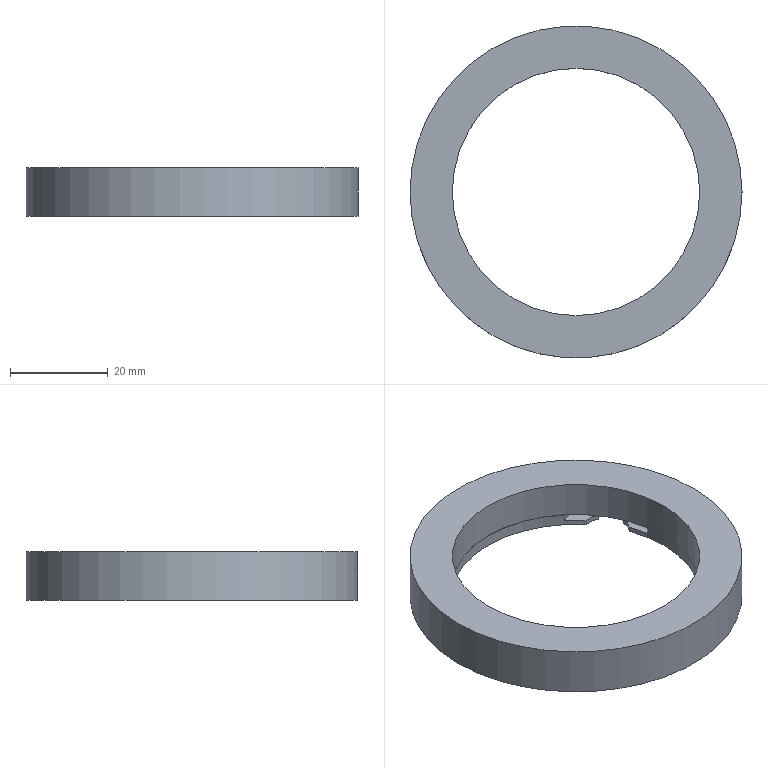Part | STEP file | 1 solid | 31 faces | box 67.8 x 67.8 x 10 mm | volume 15491 mm3 | cylinder 17 | plane 12 | cone 2 | commonest cylinder face diameters 9.7 x4 5.3 x3 17.7 x3 50.7 x3 10 x2 50.5 x1
STEP:
#1=CARTESIAN_POINT('',(-8.838,-23.759,-13.81));
#2=VERTEX_POINT('',#1);
#3=CARTESIAN_POINT('',(-8.838,-23.759,-15.31));
#4=VERTEX_POINT('',#3);
#5=CARTESIAN_POINT('',(-8.838,-23.759,-13.81));
#6=DIRECTION('',(0.,0.,-1.));
#7=VECTOR('',#6,1.);
#8=LINE('',#5,#7);
#9=EDGE_CURVE('',#2,#4,#8,.T.);
#10=ORIENTED_EDGE('',*,*,#9,.F.);
#11=CARTESIAN_POINT('',(8.838,-23.759,-13.81));
#12=VERTEX_POINT('',#11);
#13=CARTESIAN_POINT('',(0.,-23.3,-13.81));
#14=DIRECTION('',(0.,0.,-1.));
#15=DIRECTION('',(0.9987,-0.05191,0.));
#16=AXIS2_PLACEMENT_3D('',#13,#14,#15);
#17=CIRCLE('',#16,8.85);
#18=EDGE_CURVE('',#12,#2,#17,.T.);
#19=ORIENTED_EDGE('',*,*,#18,.F.);
#20=CARTESIAN_POINT('',(8.838,-23.759,-15.31));
#21=VERTEX_POINT('',#20);
#22=CARTESIAN_POINT('',(8.838,-23.759,-15.31));
#23=DIRECTION('',(0.,0.,1.));
#24=VECTOR('',#23,1.);
#25=LINE('',#22,#24);
#26=EDGE_CURVE('',#21,#12,#25,.T.);
#27=ORIENTED_EDGE('',*,*,#26,.F.);
#28=CARTESIAN_POINT('',(0.,-23.3,-15.31));
#29=DIRECTION('',(0.,0.,1.));
#30=DIRECTION('',(-0.9987,-0.05191,0.));
#31=AXIS2_PLACEMENT_3D('',#28,#29,#30);
#32=CIRCLE('',#31,8.85);
#33=EDGE_CURVE('',#4,#21,#32,.T.);
#34=ORIENTED_EDGE('',*,*,#33,.F.);
#35=EDGE_LOOP('',(#10,#19,#27,#34));
#36=FACE_BOUND('',#35,.T.);
#37=CARTESIAN_POINT('',(0.,-23.3,-15.31));
#38=DIRECTION('',(0.,0.,-1.));
#39=DIRECTION('',(0.,-1.,0.));
#40=AXIS2_PLACEMENT_3D('',#37,#38,#39);
#41=CYLINDRICAL_SURFACE('',#40,8.85);
#42=ADVANCED_FACE('',(#36),#41,.F.);
#43=CARTESIAN_POINT('',(4.736,-24.904,-16.31));
#44=VERTEX_POINT('',#43);
#45=CARTESIAN_POINT('',(4.736,-24.904,-15.31));
#46=VERTEX_POINT('',#45);
#47=CARTESIAN_POINT('',(4.736,-24.904,-16.31));
#48=DIRECTION('',(0.,0.,1.));
#49=VECTOR('',#48,1.);
#50=LINE('',#47,#49);
#51=EDGE_CURVE('',#44,#46,#50,.T.);
#52=ORIENTED_EDGE('',*,*,#51,.T.);
#53=CARTESIAN_POINT('',(0.,0.,-15.31));
#54=DIRECTION('',(0.,0.,-1.));
#55=DIRECTION('',(0.3486,-0.9373,0.));
#56=AXIS2_PLACEMENT_3D('',#53,#54,#55);
#57=CIRCLE('',#56,25.35);
#58=EDGE_CURVE('',#21,#46,#57,.T.);
#59=ORIENTED_EDGE('',*,*,#58,.F.);
#60=ORIENTED_EDGE('',*,*,#26,.T.);
#61=CARTESIAN_POINT('',(24.995,4.226,-13.81));
#62=VERTEX_POINT('',#61);
#63=CARTESIAN_POINT('',(0.,0.,-13.81));
#64=DIRECTION('',(0.,0.,-1.));
#65=DIRECTION('',(0.986,0.1667,0.));
#66=AXIS2_PLACEMENT_3D('',#63,#64,#65);
#67=CIRCLE('',#66,25.35);
#68=EDGE_CURVE('',#62,#12,#67,.T.);
#69=ORIENTED_EDGE('',*,*,#68,.F.);
#70=CARTESIAN_POINT('',(24.995,4.226,-15.31));
#71=VERTEX_POINT('',#70);
#72=CARTESIAN_POINT('',(24.995,4.226,-13.81));
#73=DIRECTION('',(0.,0.,-1.));
#74=VECTOR('',#73,1.);
#75=LINE('',#72,#74);
#76=EDGE_CURVE('',#62,#71,#75,.T.);
#77=ORIENTED_EDGE('',*,*,#76,.T.);
#78=CARTESIAN_POINT('',(23.878,8.513,-15.31));
#79=VERTEX_POINT('',#78);
#80=CARTESIAN_POINT('',(0.,0.,-15.31));
#81=DIRECTION('',(0.,0.,-1.));
#82=DIRECTION('',(0.9419,0.3358,0.));
#83=AXIS2_PLACEMENT_3D('',#80,#81,#82);
#84=CIRCLE('',#83,25.35);
#85=EDGE_CURVE('',#79,#71,#84,.T.);
#86=ORIENTED_EDGE('',*,*,#85,.F.);
#87=CARTESIAN_POINT('',(23.878,8.513,-16.31));
#88=VERTEX_POINT('',#87);
#89=CARTESIAN_POINT('',(23.878,8.513,-15.31));
#90=DIRECTION('',(0.,0.,-1.));
#91=VECTOR('',#90,1.);
#92=LINE('',#89,#91);
#93=EDGE_CURVE('',#79,#88,#92,.T.);
#94=ORIENTED_EDGE('',*,*,#93,.T.);
#95=CARTESIAN_POINT('',(0.,0.,-16.31));
#96=DIRECTION('',(0.,0.,1.));
#97=DIRECTION('',(0.1868,-0.9824,0.));
#98=AXIS2_PLACEMENT_3D('',#95,#96,#97);
#99=CIRCLE('',#98,25.35);
#100=EDGE_CURVE('',#44,#88,#99,.T.);
#101=ORIENTED_EDGE('',*,*,#100,.F.);
#102=EDGE_LOOP('',(#52,#59,#60,#69,#77,#86,#94,#101));
#103=FACE_BOUND('',#102,.T.);
#104=CARTESIAN_POINT('',(0.,0.,-16.31));
#105=DIRECTION('',(0.,0.,-1.));
#106=DIRECTION('',(0.5,-0.866,0.));
#107=AXIS2_PLACEMENT_3D('',#104,#105,#106);
#108=CYLINDRICAL_SURFACE('',#107,25.35);
#109=ADVANCED_FACE('',(#103),#108,.F.);
#110=CARTESIAN_POINT('',(16.157,19.534,-15.31));
#111=VERTEX_POINT('',#110);
#112=CARTESIAN_POINT('',(16.157,19.534,-13.81));
#113=VERTEX_POINT('',#112);
#114=CARTESIAN_POINT('',(16.157,19.534,-15.31));
#115=DIRECTION('',(0.,0.,1.));
#116=VECTOR('',#115,1.);
#117=LINE('',#114,#116);
#118=EDGE_CURVE('',#111,#113,#117,.T.);
#119=ORIENTED_EDGE('',*,*,#118,.F.);
#120=CARTESIAN_POINT('',(20.178,11.65,-15.31));
#121=DIRECTION('',(0.,0.,1.));
#122=DIRECTION('',(0.5443,-0.8389,0.));
#123=AXIS2_PLACEMENT_3D('',#120,#121,#122);
#124=CIRCLE('',#123,8.85);
#125=EDGE_CURVE('',#71,#111,#124,.T.);
#126=ORIENTED_EDGE('',*,*,#125,.F.);
#127=ORIENTED_EDGE('',*,*,#76,.F.);
#128=CARTESIAN_POINT('',(20.178,11.65,-13.81));
#129=DIRECTION('',(0.,0.,-1.));
#130=DIRECTION('',(-0.4544,0.8908,0.));
#131=AXIS2_PLACEMENT_3D('',#128,#129,#130);
#132=CIRCLE('',#131,8.85);
#133=EDGE_CURVE('',#113,#62,#132,.T.);
#134=ORIENTED_EDGE('',*,*,#133,.F.);
#135=EDGE_LOOP('',(#119,#126,#127,#134));
#136=FACE_BOUND('',#135,.T.);
#137=CARTESIAN_POINT('',(20.178,11.65,-15.31));
#138=DIRECTION('',(0.,0.,1.));
#139=DIRECTION('',(0.866,0.5,0.));
#140=AXIS2_PLACEMENT_3D('',#137,#138,#139);
#141=CYLINDRICAL_SURFACE('',#140,8.85);
#142=ADVANCED_FACE('',(#136),#141,.F.);
#143=CARTESIAN_POINT('',(-16.157,19.534,-13.81));
#144=VERTEX_POINT('',#143);
#145=CARTESIAN_POINT('',(-16.157,19.534,-15.31));
#146=VERTEX_POINT('',#145);
#147=CARTESIAN_POINT('',(-16.157,19.534,-13.81));
#148=DIRECTION('',(0.,0.,-1.));
#149=VECTOR('',#148,1.);
#150=LINE('',#147,#149);
#151=EDGE_CURVE('',#144,#146,#150,.T.);
#152=ORIENTED_EDGE('',*,*,#151,.T.);
#153=CARTESIAN_POINT('',(-19.312,16.422,-15.31));
#154=VERTEX_POINT('',#153);
#155=CARTESIAN_POINT('',(0.,0.,-15.31));
#156=DIRECTION('',(0.,0.,-1.));
#157=DIRECTION('',(-0.7618,0.6478,0.));
#158=AXIS2_PLACEMENT_3D('',#155,#156,#157);
#159=CIRCLE('',#158,25.35);
#160=EDGE_CURVE('',#154,#146,#159,.T.);
#161=ORIENTED_EDGE('',*,*,#160,.F.);
#162=CARTESIAN_POINT('',(-19.312,16.422,-16.31));
#163=VERTEX_POINT('',#162);
#164=CARTESIAN_POINT('',(-19.312,16.422,-15.31));
#165=DIRECTION('',(0.,0.,-1.));
#166=VECTOR('',#165,1.);
#167=LINE('',#164,#166);
#168=EDGE_CURVE('',#154,#163,#167,.T.);
#169=ORIENTED_EDGE('',*,*,#168,.T.);
#170=CARTESIAN_POINT('',(19.312,16.422,-16.31));
#171=VERTEX_POINT('',#170);
#172=CARTESIAN_POINT('',(0.,0.,-16.31));
#173=DIRECTION('',(0.,0.,1.));
#174=DIRECTION('',(0.7618,0.6478,0.));
#175=AXIS2_PLACEMENT_3D('',#172,#173,#174);
#176=CIRCLE('',#175,25.35);
#177=EDGE_CURVE('',#171,#163,#176,.T.);
#178=ORIENTED_EDGE('',*,*,#177,.F.);
#179=CARTESIAN_POINT('',(19.312,16.422,-15.31));
#180=VERTEX_POINT('',#179);
#181=CARTESIAN_POINT('',(19.312,16.422,-16.31));
#182=DIRECTION('',(0.,0.,1.));
#183=VECTOR('',#182,1.);
#184=LINE('',#181,#183);
#185=EDGE_CURVE('',#171,#180,#184,.T.);
#186=ORIENTED_EDGE('',*,*,#185,.T.);
#187=CARTESIAN_POINT('',(0.,0.,-15.31));
#188=DIRECTION('',(0.,0.,-1.));
#189=DIRECTION('',(0.6374,0.7706,0.));
#190=AXIS2_PLACEMENT_3D('',#187,#188,#189);
#191=CIRCLE('',#190,25.35);
#192=EDGE_CURVE('',#111,#180,#191,.T.);
#193=ORIENTED_EDGE('',*,*,#192,.F.);
#194=ORIENTED_EDGE('',*,*,#118,.T.);
#195=CARTESIAN_POINT('',(0.,0.,-13.81));
#196=DIRECTION('',(0.,0.,-1.));
#197=DIRECTION('',(-0.6374,0.7706,0.));
#198=AXIS2_PLACEMENT_3D('',#195,#196,#197);
#199=CIRCLE('',#198,25.35);
#200=EDGE_CURVE('',#144,#113,#199,.T.);
#201=ORIENTED_EDGE('',*,*,#200,.F.);
#202=EDGE_LOOP('',(#152,#161,#169,#178,#186,#193,#194,#201));
#203=FACE_BOUND('',#202,.T.);
#204=CARTESIAN_POINT('',(0.,0.,-16.31));
#205=DIRECTION('',(0.,0.,-1.));
#206=DIRECTION('',(0.5,-0.866,0.));
#207=AXIS2_PLACEMENT_3D('',#204,#205,#206);
#208=CYLINDRICAL_SURFACE('',#207,25.35);
#209=ADVANCED_FACE('',(#203),#208,.F.);
#210=ORIENTED_EDGE('',*,*,#151,.F.);
#211=CARTESIAN_POINT('',(-24.995,4.226,-13.81));
#212=VERTEX_POINT('',#211);
#213=CARTESIAN_POINT('',(-20.178,11.65,-13.81));
#214=DIRECTION('',(0.,0.,-1.));
#215=DIRECTION('',(-0.5443,-0.8389,0.));
#216=AXIS2_PLACEMENT_3D('',#213,#214,#215);
#217=CIRCLE('',#216,8.85);
#218=EDGE_CURVE('',#212,#144,#217,.T.);
#219=ORIENTED_EDGE('',*,*,#218,.F.);
#220=CARTESIAN_POINT('',(-24.995,4.226,-15.31));
#221=VERTEX_POINT('',#220);
#222=CARTESIAN_POINT('',(-24.995,4.226,-15.31));
#223=DIRECTION('',(0.,0.,1.));
#224=VECTOR('',#223,1.);
#225=LINE('',#222,#224);
#226=EDGE_CURVE('',#221,#212,#225,.T.);
#227=ORIENTED_EDGE('',*,*,#226,.F.);
#228=CARTESIAN_POINT('',(-20.178,11.65,-15.31));
#229=DIRECTION('',(0.,0.,1.));
#230=DIRECTION('',(0.4544,0.8908,0.));
#231=AXIS2_PLACEMENT_3D('',#228,#229,#230);
#232=CIRCLE('',#231,8.85);
#233=EDGE_CURVE('',#146,#221,#232,.T.);
#234=ORIENTED_EDGE('',*,*,#233,.F.);
#235=EDGE_LOOP('',(#210,#219,#227,#234));
#236=FACE_BOUND('',#235,.T.);
#237=CARTESIAN_POINT('',(-20.178,11.65,-15.31));
#238=DIRECTION('',(0.,0.,-1.));
#239=DIRECTION('',(-0.866,0.5,0.));
#240=AXIS2_PLACEMENT_3D('',#237,#238,#239);
#241=CYLINDRICAL_SURFACE('',#240,8.85);
#242=ADVANCED_FACE('',(#236),#241,.F.);
#243=CARTESIAN_POINT('',(-16.95,29.358,-16.31));
#244=VERTEX_POINT('',#243);
#245=CARTESIAN_POINT('',(0.,0.,-16.31));
#246=DIRECTION('',(0.,0.,-1.));
#247=DIRECTION('',(0.5,-0.866,0.));
#248=AXIS2_PLACEMENT_3D('',#245,#246,#247);
#249=CIRCLE('',#248,33.9);
#250=EDGE_CURVE('',#244,#244,#249,.T.);
#251=ORIENTED_EDGE('',*,*,#250,.T.);
#252=EDGE_LOOP('',(#251));
#253=FACE_BOUND('',#252,.T.);
#254=CARTESIAN_POINT('',(-23.92,16.87,-16.31));
#255=VERTEX_POINT('',#254);
#256=CARTESIAN_POINT('',(-26.57,12.28,-16.31));
#257=VERTEX_POINT('',#256);
#258=CARTESIAN_POINT('',(-25.245,14.575,-16.31));
#259=DIRECTION('',(0.,0.,1.));
#260=DIRECTION('',(0.5,0.866,0.));
#261=AXIS2_PLACEMENT_3D('',#258,#259,#260);
#262=CIRCLE('',#261,2.65);
#263=EDGE_CURVE('',#255,#257,#262,.T.);
#264=ORIENTED_EDGE('',*,*,#263,.T.);
#265=CARTESIAN_POINT('',(-25.021,11.386,-16.31));
#266=VERTEX_POINT('',#265);
#267=CARTESIAN_POINT('',(-26.57,12.28,-16.31));
#268=DIRECTION('',(0.866,-0.5,0.));
#269=VECTOR('',#268,1.);
#270=LINE('',#267,#269);
#271=EDGE_CURVE('',#257,#266,#270,.T.);
#272=ORIENTED_EDGE('',*,*,#271,.T.);
#273=CARTESIAN_POINT('',(-23.878,8.513,-16.31));
#274=VERTEX_POINT('',#273);
#275=CARTESIAN_POINT('',(-20.178,11.65,-16.31));
#276=DIRECTION('',(0.,0.,1.));
#277=DIRECTION('',(-0.9985,-0.05442,0.));
#278=AXIS2_PLACEMENT_3D('',#275,#276,#277);
#279=CIRCLE('',#278,4.85);
#280=EDGE_CURVE('',#266,#274,#279,.T.);
#281=ORIENTED_EDGE('',*,*,#280,.T.);
#282=CARTESIAN_POINT('',(-4.736,-24.904,-16.31));
#283=VERTEX_POINT('',#282);
#284=CARTESIAN_POINT('',(0.,0.,-16.31));
#285=DIRECTION('',(0.,0.,1.));
#286=DIRECTION('',(-0.9419,0.3358,0.));
#287=AXIS2_PLACEMENT_3D('',#284,#285,#286);
#288=CIRCLE('',#287,25.35);
#289=EDGE_CURVE('',#274,#283,#288,.T.);
#290=ORIENTED_EDGE('',*,*,#289,.T.);
#291=CARTESIAN_POINT('',(-2.65,-27.54,-16.31));
#292=VERTEX_POINT('',#291);
#293=CARTESIAN_POINT('',(0.,-23.3,-16.31));
#294=DIRECTION('',(0.,0.,1.));
#295=DIRECTION('',(-0.9472,-0.3207,0.));
#296=AXIS2_PLACEMENT_3D('',#293,#294,#295);
#297=CIRCLE('',#296,5.);
#298=EDGE_CURVE('',#283,#292,#297,.T.);
#299=ORIENTED_EDGE('',*,*,#298,.T.);
#300=CARTESIAN_POINT('',(-2.65,-29.15,-16.31));
#301=VERTEX_POINT('',#300);
#302=CARTESIAN_POINT('',(-2.65,-27.54,-16.31));
#303=DIRECTION('',(0.,-1.,0.));
#304=VECTOR('',#303,1.);
#305=LINE('',#302,#304);
#306=EDGE_CURVE('',#292,#301,#305,.T.);
#307=ORIENTED_EDGE('',*,*,#306,.T.);
#308=CARTESIAN_POINT('',(2.65,-29.15,-16.31));
#309=VERTEX_POINT('',#308);
#310=CARTESIAN_POINT('',(0.,-29.15,-16.31));
#311=DIRECTION('',(0.,0.,1.));
#312=DIRECTION('',(-1.,0.,0.));
#313=AXIS2_PLACEMENT_3D('',#310,#311,#312);
#314=CIRCLE('',#313,2.65);
#315=EDGE_CURVE('',#301,#309,#314,.T.);
#316=ORIENTED_EDGE('',*,*,#315,.T.);
#317=CARTESIAN_POINT('',(2.65,-27.54,-16.31));
#318=VERTEX_POINT('',#317);
#319=CARTESIAN_POINT('',(2.65,-29.15,-16.31));
#320=DIRECTION('',(0.,1.,0.));
#321=VECTOR('',#320,1.);
#322=LINE('',#319,#321);
#323=EDGE_CURVE('',#309,#318,#322,.T.);
#324=ORIENTED_EDGE('',*,*,#323,.T.);
#325=CARTESIAN_POINT('',(0.,-23.3,-16.31));
#326=DIRECTION('',(0.,0.,1.));
#327=DIRECTION('',(0.53,-0.848,0.));
#328=AXIS2_PLACEMENT_3D('',#325,#326,#327);
#329=CIRCLE('',#328,5.);
#330=EDGE_CURVE('',#318,#44,#329,.T.);
#331=ORIENTED_EDGE('',*,*,#330,.T.);
#332=ORIENTED_EDGE('',*,*,#100,.T.);
#333=CARTESIAN_POINT('',(25.021,11.386,-16.31));
#334=VERTEX_POINT('',#333);
#335=CARTESIAN_POINT('',(20.178,11.65,-16.31));
#336=DIRECTION('',(0.,0.,1.));
#337=DIRECTION('',(0.7627,-0.6467,0.));
#338=AXIS2_PLACEMENT_3D('',#335,#336,#337);
#339=CIRCLE('',#338,4.85);
#340=EDGE_CURVE('',#88,#334,#339,.T.);
#341=ORIENTED_EDGE('',*,*,#340,.T.);
#342=CARTESIAN_POINT('',(26.57,12.28,-16.31));
#343=VERTEX_POINT('',#342);
#344=CARTESIAN_POINT('',(25.021,11.386,-16.31));
#345=DIRECTION('',(0.866,0.5,0.));
#346=VECTOR('',#345,1.);
#347=LINE('',#344,#346);
#348=EDGE_CURVE('',#334,#343,#347,.T.);
#349=ORIENTED_EDGE('',*,*,#348,.T.);
#350=CARTESIAN_POINT('',(23.92,16.87,-16.31));
#351=VERTEX_POINT('',#350);
#352=CARTESIAN_POINT('',(25.245,14.575,-16.31));
#353=DIRECTION('',(0.,0.,1.));
#354=DIRECTION('',(0.5,-0.866,0.));
#355=AXIS2_PLACEMENT_3D('',#352,#353,#354);
#356=CIRCLE('',#355,2.65);
#357=EDGE_CURVE('',#343,#351,#356,.T.);
#358=ORIENTED_EDGE('',*,*,#357,.T.);
#359=CARTESIAN_POINT('',(22.371,15.976,-16.31));
#360=VERTEX_POINT('',#359);
#361=CARTESIAN_POINT('',(23.92,16.87,-16.31));
#362=DIRECTION('',(-0.866,-0.5,0.));
#363=VECTOR('',#362,1.);
#364=LINE('',#361,#363);
#365=EDGE_CURVE('',#351,#360,#364,.T.);
#366=ORIENTED_EDGE('',*,*,#365,.T.);
#367=CARTESIAN_POINT('',(20.178,11.65,-16.31));
#368=DIRECTION('',(0.,0.,1.));
#369=DIRECTION('',(0.4521,0.892,0.));
#370=AXIS2_PLACEMENT_3D('',#367,#368,#369);
#371=CIRCLE('',#370,4.85);
#372=EDGE_CURVE('',#360,#171,#371,.T.);
#373=ORIENTED_EDGE('',*,*,#372,.T.);
#374=ORIENTED_EDGE('',*,*,#177,.T.);
#375=CARTESIAN_POINT('',(-22.371,15.976,-16.31));
#376=VERTEX_POINT('',#375);
#377=CARTESIAN_POINT('',(-20.178,11.65,-16.31));
#378=DIRECTION('',(0.,0.,1.));
#379=DIRECTION('',(0.1787,0.9839,0.));
#380=AXIS2_PLACEMENT_3D('',#377,#378,#379);
#381=CIRCLE('',#380,4.85);
#382=EDGE_CURVE('',#163,#376,#381,.T.);
#383=ORIENTED_EDGE('',*,*,#382,.T.);
#384=CARTESIAN_POINT('',(-22.371,15.976,-16.31));
#385=DIRECTION('',(-0.866,0.5,0.));
#386=VECTOR('',#385,1.);
#387=LINE('',#384,#386);
#388=EDGE_CURVE('',#376,#255,#387,.T.);
#389=ORIENTED_EDGE('',*,*,#388,.T.);
#390=EDGE_LOOP('',(#264,#272,#281,#290,#299,#307,#316,#324,#331,#332,#341,#349,#358,#366,#373,#374,#383,#389));
#391=FACE_BOUND('',#390,.T.);
#392=CARTESIAN_POINT('',(-24.595,-14.2,-16.31));
#393=VERTEX_POINT('',#392);
#394=CARTESIAN_POINT('',(-25.894,-14.95,-16.31));
#395=VERTEX_POINT('',#394);
#396=CARTESIAN_POINT('',(-25.245,-14.575,-16.31));
#397=DIRECTION('',(0.,0.,1.));
#398=DIRECTION('',(0.866,0.5,0.));
#399=AXIS2_PLACEMENT_3D('',#396,#397,#398);
#400=CIRCLE('',#399,0.75);
#401=EDGE_CURVE('',#393,#395,#400,.T.);
#402=ORIENTED_EDGE('',*,*,#401,.T.);
#403=CARTESIAN_POINT('',(-25.245,-14.575,-16.31));
#404=DIRECTION('',(0.,0.,1.));
#405=DIRECTION('',(-0.866,-0.5,0.));
#406=AXIS2_PLACEMENT_3D('',#403,#404,#405);
#407=CIRCLE('',#406,0.75);
#408=EDGE_CURVE('',#395,#393,#407,.T.);
#409=ORIENTED_EDGE('',*,*,#408,.T.);
#410=EDGE_LOOP('',(#402,#409));
#411=FACE_BOUND('',#410,.T.);
#412=CARTESIAN_POINT('',(0.,0.,-16.31));
#413=DIRECTION('',(0.,0.,1.));
#414=DIRECTION('',(1.,0.,0.));
#415=AXIS2_PLACEMENT_3D('',#412,#413,#414);
#416=PLANE('',#415);
#417=ADVANCED_FACE('',(#253,#391,#411),#416,.F.);
#418=CARTESIAN_POINT('',(-16.95,29.358,-6.31));
#419=VERTEX_POINT('',#418);
#420=CARTESIAN_POINT('',(0.,0.,-6.31));
#421=DIRECTION('',(0.,0.,1.));
#422=DIRECTION('',(-0.5,0.866,0.));
#423=AXIS2_PLACEMENT_3D('',#420,#421,#422);
#424=CIRCLE('',#423,33.9);
#425=EDGE_CURVE('',#419,#419,#424,.T.);
#426=ORIENTED_EDGE('',*,*,#425,.F.);
#427=EDGE_LOOP('',(#426));
#428=FACE_OUTER_BOUND('',#427,.T.);
#429=ORIENTED_EDGE('',*,*,#250,.F.);
#430=EDGE_LOOP('',(#429));
#431=FACE_OUTER_BOUND('',#430,.T.);
#432=CARTESIAN_POINT('',(0.,0.,-16.31));
#433=DIRECTION('',(0.,0.,-1.));
#434=DIRECTION('',(0.5,-0.866,0.));
#435=AXIS2_PLACEMENT_3D('',#432,#433,#434);
#436=CYLINDRICAL_SURFACE('',#435,33.9);
#437=ADVANCED_FACE('',(#428,#431),#436,.T.);
#438=ORIENTED_EDGE('',*,*,#425,.T.);
#439=EDGE_LOOP('',(#438));
#440=FACE_BOUND('',#439,.T.);
#441=CARTESIAN_POINT('',(21.867,12.625,-6.31));
#442=VERTEX_POINT('',#441);
#443=CARTESIAN_POINT('',(0.,0.,-6.31));
#444=DIRECTION('',(0.,0.,-1.));
#445=DIRECTION('',(-0.866,-0.5,0.));
#446=AXIS2_PLACEMENT_3D('',#443,#444,#445);
#447=CIRCLE('',#446,25.25);
#448=EDGE_CURVE('',#442,#442,#447,.T.);
#449=ORIENTED_EDGE('',*,*,#448,.T.);
#450=EDGE_LOOP('',(#449));
#451=FACE_BOUND('',#450,.T.);
#452=CARTESIAN_POINT('',(0.,0.,-6.31));
#453=DIRECTION('',(0.,0.,1.));
#454=DIRECTION('',(1.,0.,0.));
#455=AXIS2_PLACEMENT_3D('',#452,#453,#454);
#456=PLANE('',#455);
#457=ADVANCED_FACE('',(#440,#451),#456,.T.);
#458=ORIENTED_EDGE('',*,*,#448,.F.);
#459=EDGE_LOOP('',(#458));
#460=FACE_OUTER_BOUND('',#459,.T.);
#461=CARTESIAN_POINT('',(21.867,12.625,-13.81));
#462=VERTEX_POINT('',#461);
#463=CARTESIAN_POINT('',(0.,0.,-13.81));
#464=DIRECTION('',(0.,0.,1.));
#465=DIRECTION('',(0.866,0.5,0.));
#466=AXIS2_PLACEMENT_3D('',#463,#464,#465);
#467=CIRCLE('',#466,25.25);
#468=EDGE_CURVE('',#462,#462,#467,.T.);
#469=ORIENTED_EDGE('',*,*,#468,.F.);
#470=EDGE_LOOP('',(#469));
#471=FACE_OUTER_BOUND('',#470,.T.);
#472=CARTESIAN_POINT('',(0.,0.,-13.81));
#473=DIRECTION('',(0.,0.,1.));
#474=DIRECTION('',(-0.866,-0.5,0.));
#475=AXIS2_PLACEMENT_3D('',#472,#473,#474);
#476=CYLINDRICAL_SURFACE('',#475,25.25);
#477=ADVANCED_FACE('',(#460,#471),#476,.F.);
#478=ORIENTED_EDGE('',*,*,#200,.T.);
#479=ORIENTED_EDGE('',*,*,#133,.T.);
#480=ORIENTED_EDGE('',*,*,#68,.T.);
#481=ORIENTED_EDGE('',*,*,#18,.T.);
#482=CARTESIAN_POINT('',(0.,0.,-13.81));
#483=DIRECTION('',(0.,0.,-1.));
#484=DIRECTION('',(-0.3486,-0.9373,0.));
#485=AXIS2_PLACEMENT_3D('',#482,#483,#484);
#486=CIRCLE('',#485,25.35);
#487=EDGE_CURVE('',#2,#212,#486,.T.);
#488=ORIENTED_EDGE('',*,*,#487,.T.);
#489=ORIENTED_EDGE('',*,*,#218,.T.);
#490=EDGE_LOOP('',(#478,#479,#480,#481,#488,#489));
#491=FACE_BOUND('',#490,.T.);
#492=ORIENTED_EDGE('',*,*,#468,.T.);
#493=EDGE_LOOP('',(#492));
#494=FACE_BOUND('',#493,.T.);
#495=CARTESIAN_POINT('',(0.,0.,-13.81));
#496=DIRECTION('',(0.,0.,-1.));
#497=DIRECTION('',(0.,-1.,0.));
#498=AXIS2_PLACEMENT_3D('',#495,#496,#497);
#499=PLANE('',#498);
#500=ADVANCED_FACE('',(#491,#494),#499,.T.);
#501=CARTESIAN_POINT('',(25.021,11.386,-15.31));
#502=VERTEX_POINT('',#501);
#503=CARTESIAN_POINT('',(20.178,11.65,-15.31));
#504=DIRECTION('',(0.,0.,-1.));
#505=DIRECTION('',(0.9985,-0.05442,0.));
#506=AXIS2_PLACEMENT_3D('',#503,#504,#505);
#507=CIRCLE('',#506,4.85);
#508=EDGE_CURVE('',#502,#79,#507,.T.);
#509=ORIENTED_EDGE('',*,*,#508,.T.);
#510=ORIENTED_EDGE('',*,*,#85,.T.);
#511=ORIENTED_EDGE('',*,*,#125,.T.);
#512=ORIENTED_EDGE('',*,*,#192,.T.);
#513=CARTESIAN_POINT('',(22.371,15.976,-15.31));
#514=VERTEX_POINT('',#513);
#515=CARTESIAN_POINT('',(20.178,11.65,-15.31));
#516=DIRECTION('',(0.,0.,-1.));
#517=DIRECTION('',(-0.1787,0.9839,0.));
#518=AXIS2_PLACEMENT_3D('',#515,#516,#517);
#519=CIRCLE('',#518,4.85);
#520=EDGE_CURVE('',#180,#514,#519,.T.);
#521=ORIENTED_EDGE('',*,*,#520,.T.);
#522=CARTESIAN_POINT('',(23.92,16.87,-15.31));
#523=VERTEX_POINT('',#522);
#524=CARTESIAN_POINT('',(22.371,15.976,-15.31));
#525=DIRECTION('',(0.866,0.5,0.));
#526=VECTOR('',#525,1.);
#527=LINE('',#524,#526);
#528=EDGE_CURVE('',#514,#523,#527,.T.);
#529=ORIENTED_EDGE('',*,*,#528,.T.);
#530=CARTESIAN_POINT('',(26.57,12.28,-15.31));
#531=VERTEX_POINT('',#530);
#532=CARTESIAN_POINT('',(25.245,14.575,-15.31));
#533=DIRECTION('',(0.,0.,-1.));
#534=DIRECTION('',(-0.5,0.866,0.));
#535=AXIS2_PLACEMENT_3D('',#532,#533,#534);
#536=CIRCLE('',#535,2.65);
#537=EDGE_CURVE('',#523,#531,#536,.T.);
#538=ORIENTED_EDGE('',*,*,#537,.T.);
#539=CARTESIAN_POINT('',(26.57,12.28,-15.31));
#540=DIRECTION('',(-0.866,-0.5,0.));
#541=VECTOR('',#540,1.);
#542=LINE('',#539,#541);
#543=EDGE_CURVE('',#531,#502,#542,.T.);
#544=ORIENTED_EDGE('',*,*,#543,.T.);
#545=EDGE_LOOP('',(#509,#510,#511,#512,#521,#529,#538,#544));
#546=FACE_BOUND('',#545,.T.);
#547=CARTESIAN_POINT('',(0.,0.,-15.31));
#548=DIRECTION('',(0.,0.,-1.));
#549=DIRECTION('',(0.,-1.,0.));
#550=AXIS2_PLACEMENT_3D('',#547,#548,#549);
#551=PLANE('',#550);
#552=ADVANCED_FACE('',(#546),#551,.F.);
#553=ORIENTED_EDGE('',*,*,#348,.F.);
#554=CARTESIAN_POINT('',(25.021,11.386,-15.31));
#555=DIRECTION('',(0.,0.,-1.));
#556=VECTOR('',#555,1.);
#557=LINE('',#554,#556);
#558=EDGE_CURVE('',#502,#334,#557,.T.);
#559=ORIENTED_EDGE('',*,*,#558,.F.);
#560=ORIENTED_EDGE('',*,*,#543,.F.);
#561=CARTESIAN_POINT('',(26.57,12.28,-16.31));
#562=DIRECTION('',(0.,0.,1.));
#563=VECTOR('',#562,1.);
#564=LINE('',#561,#563);
#565=EDGE_CURVE('',#343,#531,#564,.T.);
#566=ORIENTED_EDGE('',*,*,#565,.F.);
#567=EDGE_LOOP('',(#553,#559,#560,#566));
#568=FACE_BOUND('',#567,.T.);
#569=CARTESIAN_POINT('',(26.57,12.28,-16.31));
#570=DIRECTION('',(0.5,-0.866,0.));
#571=DIRECTION('',(0.,0.,-1.));
#572=AXIS2_PLACEMENT_3D('',#569,#570,#571);
#573=PLANE('',#572);
#574=ADVANCED_FACE('',(#568),#573,.F.);
#575=ORIENTED_EDGE('',*,*,#357,.F.);
#576=ORIENTED_EDGE('',*,*,#565,.T.);
#577=ORIENTED_EDGE('',*,*,#537,.F.);
#578=CARTESIAN_POINT('',(23.92,16.87,-15.31));
#579=DIRECTION('',(0.,0.,-1.));
#580=VECTOR('',#579,1.);
#581=LINE('',#578,#580);
#582=EDGE_CURVE('',#523,#351,#581,.T.);
#583=ORIENTED_EDGE('',*,*,#582,.T.);
#584=EDGE_LOOP('',(#575,#576,#577,#583));
#585=FACE_BOUND('',#584,.T.);
#586=CARTESIAN_POINT('',(25.245,14.575,-16.31));
#587=DIRECTION('',(0.,0.,1.));
#588=DIRECTION('',(-0.5,0.866,0.));
#589=AXIS2_PLACEMENT_3D('',#586,#587,#588);
#590=CYLINDRICAL_SURFACE('',#589,2.65);
#591=ADVANCED_FACE('',(#585),#590,.F.);
#592=ORIENTED_EDGE('',*,*,#365,.F.);
#593=ORIENTED_EDGE('',*,*,#582,.F.);
#594=ORIENTED_EDGE('',*,*,#528,.F.);
#595=CARTESIAN_POINT('',(22.371,15.976,-16.31));
#596=DIRECTION('',(0.,0.,1.));
#597=VECTOR('',#596,1.);
#598=LINE('',#595,#597);
#599=EDGE_CURVE('',#360,#514,#598,.T.);
#600=ORIENTED_EDGE('',*,*,#599,.F.);
#601=EDGE_LOOP('',(#592,#593,#594,#600));
#602=FACE_BOUND('',#601,.T.);
#603=CARTESIAN_POINT('',(20.508,14.901,-16.31));
#604=DIRECTION('',(-0.5,0.866,0.));
#605=DIRECTION('',(0.,0.,1.));
#606=AXIS2_PLACEMENT_3D('',#603,#604,#605);
#607=PLANE('',#606);
#608=ADVANCED_FACE('',(#602),#607,.F.);
#609=ORIENTED_EDGE('',*,*,#372,.F.);
#610=ORIENTED_EDGE('',*,*,#599,.T.);
#611=ORIENTED_EDGE('',*,*,#520,.F.);
#612=ORIENTED_EDGE('',*,*,#185,.F.);
#613=EDGE_LOOP('',(#609,#610,#611,#612));
#614=FACE_BOUND('',#613,.T.);
#615=CARTESIAN_POINT('',(20.178,11.65,-16.31));
#616=DIRECTION('',(0.,0.,1.));
#617=DIRECTION('',(-0.866,-0.5,0.));
#618=AXIS2_PLACEMENT_3D('',#615,#616,#617);
#619=CYLINDRICAL_SURFACE('',#618,4.85);
#620=ADVANCED_FACE('',(#614),#619,.F.);
#621=ORIENTED_EDGE('',*,*,#340,.F.);
#622=ORIENTED_EDGE('',*,*,#93,.F.);
#623=ORIENTED_EDGE('',*,*,#508,.F.);
#624=ORIENTED_EDGE('',*,*,#558,.T.);
#625=EDGE_LOOP('',(#621,#622,#623,#624));
#626=FACE_BOUND('',#625,.T.);
#627=CARTESIAN_POINT('',(20.178,11.65,-16.31));
#628=DIRECTION('',(0.,0.,1.));
#629=DIRECTION('',(-0.866,-0.5,0.));
#630=AXIS2_PLACEMENT_3D('',#627,#628,#629);
#631=CYLINDRICAL_SURFACE('',#630,4.85);
#632=ADVANCED_FACE('',(#626),#631,.F.);
#633=CARTESIAN_POINT('',(-4.736,-24.904,-15.31));
#634=VERTEX_POINT('',#633);
#635=CARTESIAN_POINT('',(0.,0.,-15.31));
#636=DIRECTION('',(0.,0.,-1.));
#637=DIRECTION('',(-0.1868,-0.9824,0.));
#638=AXIS2_PLACEMENT_3D('',#635,#636,#637);
#639=CIRCLE('',#638,25.35);
#640=EDGE_CURVE('',#634,#4,#639,.T.);
#641=ORIENTED_EDGE('',*,*,#640,.F.);
#642=CARTESIAN_POINT('',(-4.736,-24.904,-15.31));
#643=DIRECTION('',(0.,0.,-1.));
#644=VECTOR('',#643,1.);
#645=LINE('',#642,#644);
#646=EDGE_CURVE('',#634,#283,#645,.T.);
#647=ORIENTED_EDGE('',*,*,#646,.T.);
#648=ORIENTED_EDGE('',*,*,#289,.F.);
#649=CARTESIAN_POINT('',(-23.878,8.513,-15.31));
#650=VERTEX_POINT('',#649);
#651=CARTESIAN_POINT('',(-23.878,8.513,-16.31));
#652=DIRECTION('',(0.,0.,1.));
#653=VECTOR('',#652,1.);
#654=LINE('',#651,#653);
#655=EDGE_CURVE('',#274,#650,#654,.T.);
#656=ORIENTED_EDGE('',*,*,#655,.T.);
#657=CARTESIAN_POINT('',(0.,0.,-15.31));
#658=DIRECTION('',(0.,0.,-1.));
#659=DIRECTION('',(-0.986,0.1667,0.));
#660=AXIS2_PLACEMENT_3D('',#657,#658,#659);
#661=CIRCLE('',#660,25.35);
#662=EDGE_CURVE('',#221,#650,#661,.T.);
#663=ORIENTED_EDGE('',*,*,#662,.F.);
#664=ORIENTED_EDGE('',*,*,#226,.T.);
#665=ORIENTED_EDGE('',*,*,#487,.F.);
#666=ORIENTED_EDGE('',*,*,#9,.T.);
#667=EDGE_LOOP('',(#641,#647,#648,#656,#663,#664,#665,#666));
#668=FACE_BOUND('',#667,.T.);
#669=CARTESIAN_POINT('',(0.,0.,-16.31));
#670=DIRECTION('',(0.,0.,-1.));
#671=DIRECTION('',(0.5,-0.866,0.));
#672=AXIS2_PLACEMENT_3D('',#669,#670,#671);
#673=CYLINDRICAL_SURFACE('',#672,25.35);
#674=ADVANCED_FACE('',(#668),#673,.F.);
#675=ORIENTED_EDGE('',*,*,#233,.T.);
#676=ORIENTED_EDGE('',*,*,#662,.T.);
#677=CARTESIAN_POINT('',(-25.021,11.386,-15.31));
#678=VERTEX_POINT('',#677);
#679=CARTESIAN_POINT('',(-20.178,11.65,-15.31));
#680=DIRECTION('',(0.,0.,-1.));
#681=DIRECTION('',(-0.7627,-0.6467,0.));
#682=AXIS2_PLACEMENT_3D('',#679,#680,#681);
#683=CIRCLE('',#682,4.85);
#684=EDGE_CURVE('',#650,#678,#683,.T.);
#685=ORIENTED_EDGE('',*,*,#684,.T.);
#686=CARTESIAN_POINT('',(-26.57,12.28,-15.31));
#687=VERTEX_POINT('',#686);
#688=CARTESIAN_POINT('',(-25.021,11.386,-15.31));
#689=DIRECTION('',(-0.866,0.5,0.));
#690=VECTOR('',#689,1.);
#691=LINE('',#688,#690);
#692=EDGE_CURVE('',#678,#687,#691,.T.);
#693=ORIENTED_EDGE('',*,*,#692,.T.);
#694=CARTESIAN_POINT('',(-23.92,16.87,-15.31));
#695=VERTEX_POINT('',#694);
#696=CARTESIAN_POINT('',(-25.245,14.575,-15.31));
#697=DIRECTION('',(0.,0.,-1.));
#698=DIRECTION('',(-0.5,-0.866,0.));
#699=AXIS2_PLACEMENT_3D('',#696,#697,#698);
#700=CIRCLE('',#699,2.65);
#701=EDGE_CURVE('',#687,#695,#700,.T.);
#702=ORIENTED_EDGE('',*,*,#701,.T.);
#703=CARTESIAN_POINT('',(-22.371,15.976,-15.31));
#704=VERTEX_POINT('',#703);
#705=CARTESIAN_POINT('',(-23.92,16.87,-15.31));
#706=DIRECTION('',(0.866,-0.5,0.));
#707=VECTOR('',#706,1.);
#708=LINE('',#705,#707);
#709=EDGE_CURVE('',#695,#704,#708,.T.);
#710=ORIENTED_EDGE('',*,*,#709,.T.);
#711=CARTESIAN_POINT('',(-20.178,11.65,-15.31));
#712=DIRECTION('',(0.,0.,-1.));
#713=DIRECTION('',(-0.4521,0.892,0.));
#714=AXIS2_PLACEMENT_3D('',#711,#712,#713);
#715=CIRCLE('',#714,4.85);
#716=EDGE_CURVE('',#704,#154,#715,.T.);
#717=ORIENTED_EDGE('',*,*,#716,.T.);
#718=ORIENTED_EDGE('',*,*,#160,.T.);
#719=EDGE_LOOP('',(#675,#676,#685,#693,#702,#710,#717,#718));
#720=FACE_BOUND('',#719,.T.);
#721=CARTESIAN_POINT('',(0.,0.,-15.31));
#722=DIRECTION('',(0.,0.,1.));
#723=DIRECTION('',(1.,0.,0.));
#724=AXIS2_PLACEMENT_3D('',#721,#722,#723);
#725=PLANE('',#724);
#726=ADVANCED_FACE('',(#720),#725,.T.);
#727=ORIENTED_EDGE('',*,*,#382,.F.);
#728=ORIENTED_EDGE('',*,*,#168,.F.);
#729=ORIENTED_EDGE('',*,*,#716,.F.);
#730=CARTESIAN_POINT('',(-22.371,15.976,-15.31));
#731=DIRECTION('',(0.,0.,-1.));
#732=VECTOR('',#731,1.);
#733=LINE('',#730,#732);
#734=EDGE_CURVE('',#704,#376,#733,.T.);
#735=ORIENTED_EDGE('',*,*,#734,.T.);
#736=EDGE_LOOP('',(#727,#728,#729,#735));
#737=FACE_BOUND('',#736,.T.);
#738=CARTESIAN_POINT('',(-20.178,11.65,-16.31));
#739=DIRECTION('',(0.,0.,-1.));
#740=DIRECTION('',(0.866,-0.5,0.));
#741=AXIS2_PLACEMENT_3D('',#738,#739,#740);
#742=CYLINDRICAL_SURFACE('',#741,4.85);
#743=ADVANCED_FACE('',(#737),#742,.F.);
#744=ORIENTED_EDGE('',*,*,#388,.F.);
#745=ORIENTED_EDGE('',*,*,#734,.F.);
#746=ORIENTED_EDGE('',*,*,#709,.F.);
#747=CARTESIAN_POINT('',(-23.92,16.87,-16.31));
#748=DIRECTION('',(0.,0.,1.));
#749=VECTOR('',#748,1.);
#750=LINE('',#747,#749);
#751=EDGE_CURVE('',#255,#695,#750,.T.);
#752=ORIENTED_EDGE('',*,*,#751,.F.);
#753=EDGE_LOOP('',(#744,#745,#746,#752));
#754=FACE_BOUND('',#753,.T.);
#755=CARTESIAN_POINT('',(-20.508,14.901,-16.31));
#756=DIRECTION('',(-0.5,-0.866,0.));
#757=DIRECTION('',(-0.866,0.5,0.));
#758=AXIS2_PLACEMENT_3D('',#755,#756,#757);
#759=PLANE('',#758);
#760=ADVANCED_FACE('',(#754),#759,.T.);
#761=ORIENTED_EDGE('',*,*,#263,.F.);
#762=ORIENTED_EDGE('',*,*,#751,.T.);
#763=ORIENTED_EDGE('',*,*,#701,.F.);
#764=CARTESIAN_POINT('',(-26.57,12.28,-15.31));
#765=DIRECTION('',(0.,0.,-1.));
#766=VECTOR('',#765,1.);
#767=LINE('',#764,#766);
#768=EDGE_CURVE('',#687,#257,#767,.T.);
#769=ORIENTED_EDGE('',*,*,#768,.T.);
#770=EDGE_LOOP('',(#761,#762,#763,#769));
#771=FACE_BOUND('',#770,.T.);
#772=CARTESIAN_POINT('',(-25.245,14.575,-16.31));
#773=DIRECTION('',(0.,0.,-1.));
#774=DIRECTION('',(0.5,0.866,0.));
#775=AXIS2_PLACEMENT_3D('',#772,#773,#774);
#776=CYLINDRICAL_SURFACE('',#775,2.65);
#777=ADVANCED_FACE('',(#771),#776,.F.);
#778=ORIENTED_EDGE('',*,*,#271,.F.);
#779=ORIENTED_EDGE('',*,*,#768,.F.);
#780=ORIENTED_EDGE('',*,*,#692,.F.);
#781=CARTESIAN_POINT('',(-25.021,11.386,-16.31));
#782=DIRECTION('',(0.,0.,1.));
#783=VECTOR('',#782,1.);
#784=LINE('',#781,#783);
#785=EDGE_CURVE('',#266,#678,#784,.T.);
#786=ORIENTED_EDGE('',*,*,#785,.F.);
#787=EDGE_LOOP('',(#778,#779,#780,#786));
#788=FACE_BOUND('',#787,.T.);
#789=CARTESIAN_POINT('',(-26.57,12.28,-16.31));
#790=DIRECTION('',(0.5,0.866,0.));
#791=DIRECTION('',(0.,0.,-1.));
#792=AXIS2_PLACEMENT_3D('',#789,#790,#791);
#793=PLANE('',#792);
#794=ADVANCED_FACE('',(#788),#793,.T.);
#795=ORIENTED_EDGE('',*,*,#280,.F.);
#796=ORIENTED_EDGE('',*,*,#785,.T.);
#797=ORIENTED_EDGE('',*,*,#684,.F.);
#798=ORIENTED_EDGE('',*,*,#655,.F.);
#799=EDGE_LOOP('',(#795,#796,#797,#798));
#800=FACE_BOUND('',#799,.T.);
#801=CARTESIAN_POINT('',(-20.178,11.65,-16.31));
#802=DIRECTION('',(0.,0.,-1.));
#803=DIRECTION('',(0.866,-0.5,0.));
#804=AXIS2_PLACEMENT_3D('',#801,#802,#803);
#805=CYLINDRICAL_SURFACE('',#804,4.85);
#806=ADVANCED_FACE('',(#800),#805,.F.);
#807=ORIENTED_EDGE('',*,*,#298,.F.);
#808=ORIENTED_EDGE('',*,*,#646,.F.);
#809=CARTESIAN_POINT('',(-2.65,-27.54,-15.31));
#810=VERTEX_POINT('',#809);
#811=CARTESIAN_POINT('',(0.,-23.3,-15.31));
#812=DIRECTION('',(0.,0.,-1.));
#813=DIRECTION('',(-0.53,-0.848,0.));
#814=AXIS2_PLACEMENT_3D('',#811,#812,#813);
#815=CIRCLE('',#814,5.);
#816=EDGE_CURVE('',#810,#634,#815,.T.);
#817=ORIENTED_EDGE('',*,*,#816,.F.);
#818=CARTESIAN_POINT('',(-2.65,-27.54,-15.31));
#819=DIRECTION('',(0.,0.,-1.));
#820=VECTOR('',#819,1.);
#821=LINE('',#818,#820);
#822=EDGE_CURVE('',#810,#292,#821,.T.);
#823=ORIENTED_EDGE('',*,*,#822,.T.);
#824=EDGE_LOOP('',(#807,#808,#817,#823));
#825=FACE_BOUND('',#824,.T.);
#826=CARTESIAN_POINT('',(0.,-23.3,-16.31));
#827=DIRECTION('',(0.,0.,-1.));
#828=DIRECTION('',(0.,1.,0.));
#829=AXIS2_PLACEMENT_3D('',#826,#827,#828);
#830=CYLINDRICAL_SURFACE('',#829,5.);
#831=ADVANCED_FACE('',(#825),#830,.F.);
#832=ORIENTED_EDGE('',*,*,#306,.F.);
#833=ORIENTED_EDGE('',*,*,#822,.F.);
#834=CARTESIAN_POINT('',(-2.65,-29.15,-15.31));
#835=VERTEX_POINT('',#834);
#836=CARTESIAN_POINT('',(-2.65,-29.15,-15.31));
#837=DIRECTION('',(0.,1.,0.));
#838=VECTOR('',#837,1.);
#839=LINE('',#836,#838);
#840=EDGE_CURVE('',#835,#810,#839,.T.);
#841=ORIENTED_EDGE('',*,*,#840,.F.);
#842=CARTESIAN_POINT('',(-2.65,-29.15,-16.31));
#843=DIRECTION('',(0.,0.,1.));
#844=VECTOR('',#843,1.);
#845=LINE('',#842,#844);
#846=EDGE_CURVE('',#301,#835,#845,.T.);
#847=ORIENTED_EDGE('',*,*,#846,.F.);
#848=EDGE_LOOP('',(#832,#833,#841,#847));
#849=FACE_BOUND('',#848,.T.);
#850=CARTESIAN_POINT('',(-2.65,-25.211,-16.31));
#851=DIRECTION('',(1.,0.,0.));
#852=DIRECTION('',(0.,1.,0.));
#853=AXIS2_PLACEMENT_3D('',#850,#851,#852);
#854=PLANE('',#853);
#855=ADVANCED_FACE('',(#849),#854,.T.);
#856=ORIENTED_EDGE('',*,*,#315,.F.);
#857=ORIENTED_EDGE('',*,*,#846,.T.);
#858=CARTESIAN_POINT('',(2.65,-29.15,-15.31));
#859=VERTEX_POINT('',#858);
#860=CARTESIAN_POINT('',(0.,-29.15,-15.31));
#861=DIRECTION('',(0.,0.,-1.));
#862=DIRECTION('',(1.,0.,0.));
#863=AXIS2_PLACEMENT_3D('',#860,#861,#862);
#864=CIRCLE('',#863,2.65);
#865=EDGE_CURVE('',#859,#835,#864,.T.);
#866=ORIENTED_EDGE('',*,*,#865,.F.);
#867=CARTESIAN_POINT('',(2.65,-29.15,-15.31));
#868=DIRECTION('',(0.,0.,-1.));
#869=VECTOR('',#868,1.);
#870=LINE('',#867,#869);
#871=EDGE_CURVE('',#859,#309,#870,.T.);
#872=ORIENTED_EDGE('',*,*,#871,.T.);
#873=EDGE_LOOP('',(#856,#857,#866,#872));
#874=FACE_BOUND('',#873,.T.);
#875=CARTESIAN_POINT('',(0.,-29.15,-16.31));
#876=DIRECTION('',(0.,0.,-1.));
#877=DIRECTION('',(-1.,0.,0.));
#878=AXIS2_PLACEMENT_3D('',#875,#876,#877);
#879=CYLINDRICAL_SURFACE('',#878,2.65);
#880=ADVANCED_FACE('',(#874),#879,.F.);
#881=ORIENTED_EDGE('',*,*,#323,.F.);
#882=ORIENTED_EDGE('',*,*,#871,.F.);
#883=CARTESIAN_POINT('',(2.65,-27.54,-15.31));
#884=VERTEX_POINT('',#883);
#885=CARTESIAN_POINT('',(2.65,-27.54,-15.31));
#886=DIRECTION('',(0.,-1.,0.));
#887=VECTOR('',#886,1.);
#888=LINE('',#885,#887);
#889=EDGE_CURVE('',#884,#859,#888,.T.);
#890=ORIENTED_EDGE('',*,*,#889,.F.);
#891=CARTESIAN_POINT('',(2.65,-27.54,-16.31));
#892=DIRECTION('',(0.,0.,1.));
#893=VECTOR('',#892,1.);
#894=LINE('',#891,#893);
#895=EDGE_CURVE('',#318,#884,#894,.T.);
#896=ORIENTED_EDGE('',*,*,#895,.F.);
#897=EDGE_LOOP('',(#881,#882,#890,#896));
#898=FACE_BOUND('',#897,.T.);
#899=CARTESIAN_POINT('',(2.65,-29.15,-16.31));
#900=DIRECTION('',(-1.,0.,0.));
#901=DIRECTION('',(0.,0.,1.));
#902=AXIS2_PLACEMENT_3D('',#899,#900,#901);
#903=PLANE('',#902);
#904=ADVANCED_FACE('',(#898),#903,.T.);
#905=ORIENTED_EDGE('',*,*,#330,.F.);
#906=ORIENTED_EDGE('',*,*,#895,.T.);
#907=CARTESIAN_POINT('',(0.,-23.3,-15.31));
#908=DIRECTION('',(0.,0.,-1.));
#909=DIRECTION('',(0.9472,-0.3207,0.));
#910=AXIS2_PLACEMENT_3D('',#907,#908,#909);
#911=CIRCLE('',#910,5.);
#912=EDGE_CURVE('',#46,#884,#911,.T.);
#913=ORIENTED_EDGE('',*,*,#912,.F.);
#914=ORIENTED_EDGE('',*,*,#51,.F.);
#915=EDGE_LOOP('',(#905,#906,#913,#914));
#916=FACE_BOUND('',#915,.T.);
#917=CARTESIAN_POINT('',(0.,-23.3,-16.31));
#918=DIRECTION('',(0.,0.,-1.));
#919=DIRECTION('',(0.,1.,0.));
#920=AXIS2_PLACEMENT_3D('',#917,#918,#919);
#921=CYLINDRICAL_SURFACE('',#920,5.);
#922=ADVANCED_FACE('',(#916),#921,.F.);
#923=ORIENTED_EDGE('',*,*,#33,.T.);
#924=ORIENTED_EDGE('',*,*,#58,.T.);
#925=ORIENTED_EDGE('',*,*,#912,.T.);
#926=ORIENTED_EDGE('',*,*,#889,.T.);
#927=ORIENTED_EDGE('',*,*,#865,.T.);
#928=ORIENTED_EDGE('',*,*,#840,.T.);
#929=ORIENTED_EDGE('',*,*,#816,.T.);
#930=ORIENTED_EDGE('',*,*,#640,.T.);
#931=EDGE_LOOP('',(#923,#924,#925,#926,#927,#928,#929,#930));
#932=FACE_BOUND('',#931,.T.);
#933=CARTESIAN_POINT('',(0.,0.,-15.31));
#934=DIRECTION('',(0.,0.,1.));
#935=DIRECTION('',(1.,0.,0.));
#936=AXIS2_PLACEMENT_3D('',#933,#934,#935);
#937=PLANE('',#936);
#938=ADVANCED_FACE('',(#932),#937,.T.);
#939=ORIENTED_EDGE('',*,*,#408,.F.);
#940=CARTESIAN_POINT('',(-25.245,-14.575,-15.56));
#941=VERTEX_POINT('',#940);
#942=CARTESIAN_POINT('',(-25.245,-14.575,-15.56));
#943=DIRECTION('',(-0.6124,-0.3536,-0.7071));
#944=VECTOR('',#943,1.);
#945=LINE('',#942,#944);
#946=EDGE_CURVE('',#941,#395,#945,.T.);
#947=ORIENTED_EDGE('',*,*,#946,.F.);
#948=CARTESIAN_POINT('',(-24.595,-14.2,-16.31));
#949=DIRECTION('',(-0.6124,-0.3536,0.7071));
#950=VECTOR('',#949,1.);
#951=LINE('',#948,#950);
#952=EDGE_CURVE('',#393,#941,#951,.T.);
#953=ORIENTED_EDGE('',*,*,#952,.F.);
#954=EDGE_LOOP('',(#939,#947,#953));
#955=FACE_BOUND('',#954,.T.);
#956=CARTESIAN_POINT('',(-25.245,-14.575,-15.935));
#957=DIRECTION('',(0.,0.,-1.));
#958=DIRECTION('',(-0.866,-0.5,0.));
#959=AXIS2_PLACEMENT_3D('',#956,#957,#958);
#960=CONICAL_SURFACE('',#959,0.375,0.7854);
#961=ADVANCED_FACE('',(#955),#960,.F.);
#962=ORIENTED_EDGE('',*,*,#952,.T.);
#963=ORIENTED_EDGE('',*,*,#946,.T.);
#964=ORIENTED_EDGE('',*,*,#401,.F.);
#965=EDGE_LOOP('',(#962,#963,#964));
#966=FACE_BOUND('',#965,.T.);
#967=CARTESIAN_POINT('',(-25.245,-14.575,-15.935));
#968=DIRECTION('',(0.,0.,-1.));
#969=DIRECTION('',(-0.866,-0.5,0.));
#970=AXIS2_PLACEMENT_3D('',#967,#968,#969);
#971=CONICAL_SURFACE('',#970,0.375,0.7854);
#972=ADVANCED_FACE('',(#966),#971,.F.);
#973=CLOSED_SHELL('',(#42,#109,#142,#209,#242,#417,#437,#457,#477,#500,#552,#574,#591,#608,#620,#632,#674,#726,#743,#760,#777,#794,#806,#831,#855,#880,#904,#922,#938,#961,#972));
#974=MANIFOLD_SOLID_BREP('',#973);
#975=(LENGTH_UNIT()NAMED_UNIT(*)SI_UNIT(.MILLI.,.METRE.));
#976=UNCERTAINTY_MEASURE_WITH_UNIT(LENGTH_MEASURE(0.00001),#975,'','');
#977=(NAMED_UNIT(*)PLANE_ANGLE_UNIT()SI_UNIT($,.RADIAN.));
#978=(NAMED_UNIT(*)SI_UNIT($,.STERADIAN.)SOLID_ANGLE_UNIT());
#979=(GEOMETRIC_REPRESENTATION_CONTEXT(3)GLOBAL_UNCERTAINTY_ASSIGNED_CONTEXT((#976))GLOBAL_UNIT_ASSIGNED_CONTEXT((#975,#977,#978))REPRESENTATION_CONTEXT('',''));
#980=ADVANCED_BREP_SHAPE_REPRESENTATION('',(#974),#979);